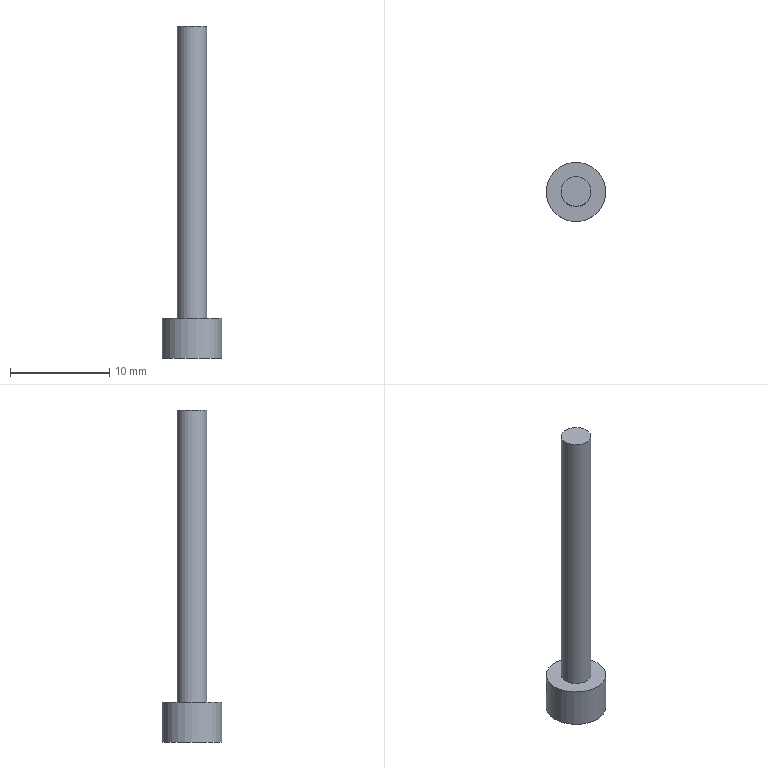Part | STEP file | 200 mesh_id1118 | 1 solid | 5 faces | box 6 x 6 x 33.5 mm | volume 321.621 mm3 | plane 3 | cylinder 2 | commonest cylinder face diameters 3 x1 6 x1
STEP:
#1=CARTESIAN_POINT('',(-17020.048,-3987.769,29.5));
#2=VERTEX_POINT('',#1);
#3=CARTESIAN_POINT('',(-17021.548,-3987.769,29.5));
#4=DIRECTION('',(0.,0.,-1.));
#5=DIRECTION('',(1.,0.,0.));
#6=AXIS2_PLACEMENT_3D('',#3,#4,#5);
#7=CIRCLE('',#6,1.5);
#8=EDGE_CURVE('',#2,#2,#7,.T.);
#9=ORIENTED_EDGE('',*,*,#8,.F.);
#10=EDGE_LOOP('',(#9));
#11=FACE_OUTER_BOUND('',#10,.T.);
#12=CARTESIAN_POINT('',(-17021.548,-3987.769,29.5));
#13=DIRECTION('',(0.,0.,1.));
#14=DIRECTION('',(1.,0.,0.));
#15=AXIS2_PLACEMENT_3D('',#12,#13,#14);
#16=PLANE('',#15);
#17=ADVANCED_FACE('',(#11),#16,.T.);
#18=ORIENTED_EDGE('',*,*,#8,.T.);
#19=EDGE_LOOP('',(#18));
#20=FACE_BOUND('',#19,.T.);
#21=CARTESIAN_POINT('',(-17020.048,-3987.769,0.));
#22=VERTEX_POINT('',#21);
#23=CARTESIAN_POINT('',(-17021.548,-3987.769,0.));
#24=DIRECTION('',(0.,0.,-1.));
#25=DIRECTION('',(1.,0.,0.));
#26=AXIS2_PLACEMENT_3D('',#23,#24,#25);
#27=CIRCLE('',#26,1.5);
#28=EDGE_CURVE('',#22,#22,#27,.T.);
#29=ORIENTED_EDGE('',*,*,#28,.F.);
#30=EDGE_LOOP('',(#29));
#31=FACE_BOUND('',#30,.T.);
#32=CARTESIAN_POINT('',(-17021.548,-3987.769,0.2));
#33=DIRECTION('',(0.,0.,1.));
#34=DIRECTION('',(1.,0.,0.));
#35=AXIS2_PLACEMENT_3D('',#32,#33,#34);
#36=CYLINDRICAL_SURFACE('',#35,1.5);
#37=ADVANCED_FACE('',(#20,#31),#36,.T.);
#38=CARTESIAN_POINT('',(-17024.548,-3987.769,-4.));
#39=VERTEX_POINT('',#38);
#40=CARTESIAN_POINT('',(-17021.548,-3987.769,-4.));
#41=DIRECTION('',(0.,0.,1.));
#42=DIRECTION('',(-1.,0.,0.));
#43=AXIS2_PLACEMENT_3D('',#40,#41,#42);
#44=CIRCLE('',#43,3.);
#45=EDGE_CURVE('',#39,#39,#44,.T.);
#46=ORIENTED_EDGE('',*,*,#45,.F.);
#47=EDGE_LOOP('',(#46));
#48=FACE_OUTER_BOUND('',#47,.T.);
#49=CARTESIAN_POINT('',(-17021.548,-3987.769,-4.));
#50=DIRECTION('',(0.,0.,-1.));
#51=DIRECTION('',(-1.,0.,0.));
#52=AXIS2_PLACEMENT_3D('',#49,#50,#51);
#53=PLANE('',#52);
#54=ADVANCED_FACE('',(#48),#53,.T.);
#55=ORIENTED_EDGE('',*,*,#28,.T.);
#56=EDGE_LOOP('',(#55));
#57=FACE_BOUND('',#56,.T.);
#58=CARTESIAN_POINT('',(-17018.548,-3987.769,0.));
#59=VERTEX_POINT('',#58);
#60=CARTESIAN_POINT('',(-17021.548,-3987.769,0.));
#61=DIRECTION('',(0.,0.,-1.));
#62=DIRECTION('',(1.,0.,0.));
#63=AXIS2_PLACEMENT_3D('',#60,#61,#62);
#64=CIRCLE('',#63,3.);
#65=EDGE_CURVE('',#59,#59,#64,.T.);
#66=ORIENTED_EDGE('',*,*,#65,.F.);
#67=EDGE_LOOP('',(#66));
#68=FACE_BOUND('',#67,.T.);
#69=CARTESIAN_POINT('',(-17021.548,-3987.769,0.));
#70=DIRECTION('',(0.,0.,1.));
#71=DIRECTION('',(1.,0.,0.));
#72=AXIS2_PLACEMENT_3D('',#69,#70,#71);
#73=PLANE('',#72);
#74=ADVANCED_FACE('',(#57,#68),#73,.T.);
#75=ORIENTED_EDGE('',*,*,#45,.T.);
#76=EDGE_LOOP('',(#75));
#77=FACE_BOUND('',#76,.T.);
#78=ORIENTED_EDGE('',*,*,#65,.T.);
#79=EDGE_LOOP('',(#78));
#80=FACE_BOUND('',#79,.T.);
#81=CARTESIAN_POINT('',(-17021.548,-3987.769,0.));
#82=DIRECTION('',(0.,0.,-1.));
#83=DIRECTION('',(1.,0.,0.));
#84=AXIS2_PLACEMENT_3D('',#81,#82,#83);
#85=CYLINDRICAL_SURFACE('',#84,3.);
#86=ADVANCED_FACE('',(#77,#80),#85,.T.);
#87=CLOSED_SHELL('',(#17,#37,#54,#74,#86));
#88=MANIFOLD_SOLID_BREP('',#87);
#89=(LENGTH_UNIT()NAMED_UNIT(*)SI_UNIT(.MILLI.,.METRE.));
#90=UNCERTAINTY_MEASURE_WITH_UNIT(LENGTH_MEASURE(0.00002),#89,'','');
#91=(NAMED_UNIT(*)PLANE_ANGLE_UNIT()SI_UNIT($,.RADIAN.));
#92=PLANE_ANGLE_MEASURE_WITH_UNIT(PLANE_ANGLE_MEASURE(0.01745),#91);
#93=DIMENSIONAL_EXPONENTS(0.,0.,0.,0.,0.,0.,0.);
#94=(CONVERSION_BASED_UNIT('DEGREE',#92)NAMED_UNIT(#93)PLANE_ANGLE_UNIT());
#95=(NAMED_UNIT(*)SI_UNIT($,.STERADIAN.)SOLID_ANGLE_UNIT());
#96=(GEOMETRIC_REPRESENTATION_CONTEXT(3)GLOBAL_UNCERTAINTY_ASSIGNED_CONTEXT((#90))GLOBAL_UNIT_ASSIGNED_CONTEXT((#89,#94,#95))REPRESENTATION_CONTEXT('',''));
#97=ADVANCED_BREP_SHAPE_REPRESENTATION('',(#88),#96);